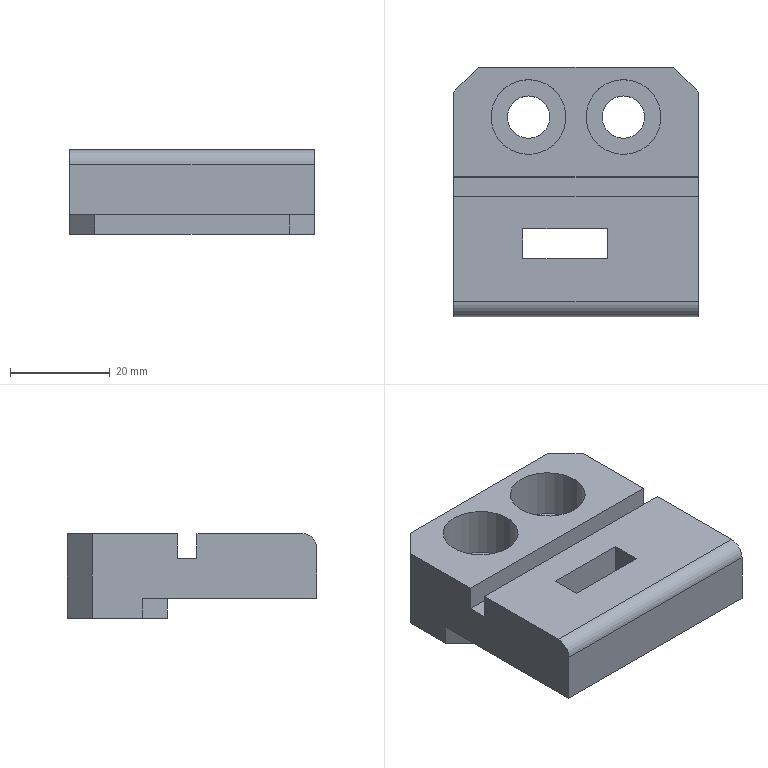Part | STEP file | gslz 2016.10.28-13_id342_x_t | 1 solid | 27 faces | box 49 x 50 x 17 mm | volume 28516 mm3 | plane 22 | cylinder 5 | commonest cylinder face diameters 8.5 x2 15 x2 6 x1